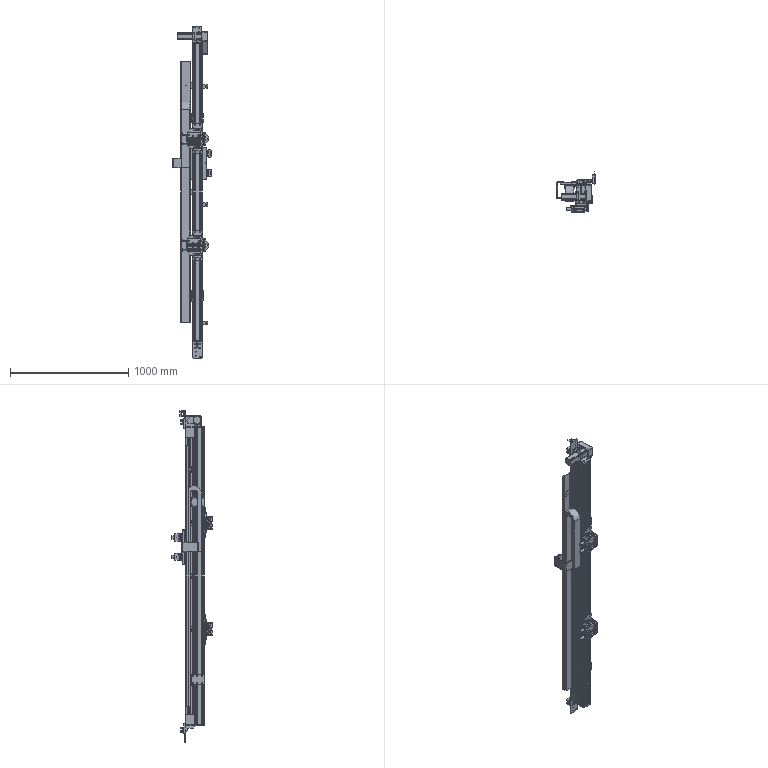Part | SolidWorks | features ReferencePattern 10, LocalLPattern 3, MirrorCompFeat 1 | 83 solids | 4934 faces | volume 30075054 mm3 | plane 2120 | cylinder 1909 | cone 490 | torus 236 | sphere 128 | spline 51 | commonest cylinder face diameters 9 x144 0.4 x128 7 x96 5 x91 6 x80 4 x66